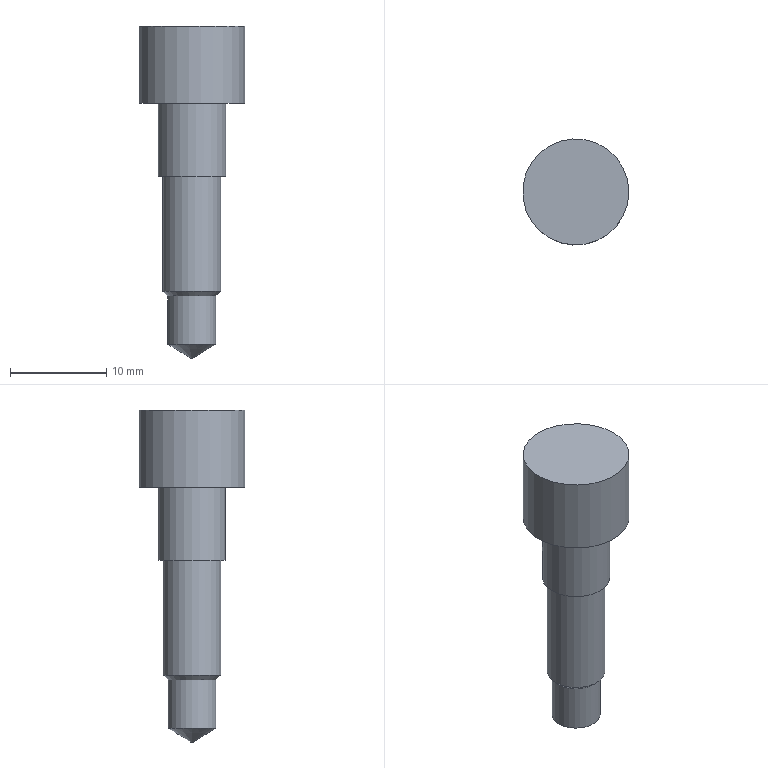Part | NX | features BREP 2 | 2 solids | 21 faces | box 11 x 11 x 34.43 mm | volume 2353 mm3 | plane 14 | cylinder 5 | cone 2 | commonest cylinder face diameters 5 x1 6 x1 7 x1 10 x1 11 x1
STEP:
#1=CARTESIAN_POINT('',(-2.5,0.,0.));
#2=VERTEX_POINT('',#1);
#3=CARTESIAN_POINT('',(0.,0.,0.));
#4=DIRECTION('',(0.,0.,1.));
#5=DIRECTION('',(-1.,0.,0.));
#6=AXIS2_PLACEMENT_3D('',#3,#4,#5);
#7=CIRCLE('',#6,2.5);
#8=EDGE_CURVE('',#2,#2,#7,.T.);
#9=ORIENTED_EDGE('',*,*,#8,.F.);
#10=EDGE_LOOP('',(#9));
#11=FACE_BOUND('',#10,.T.);
#12=CARTESIAN_POINT('',(-2.5,0.,-17.4));
#13=VERTEX_POINT('',#12);
#14=CARTESIAN_POINT('',(0.,0.,-17.4));
#15=DIRECTION('',(0.,0.,-1.));
#16=DIRECTION('',(-1.,0.,0.));
#17=AXIS2_PLACEMENT_3D('',#14,#15,#16);
#18=CIRCLE('',#17,2.5);
#19=EDGE_CURVE('',#13,#13,#18,.T.);
#20=ORIENTED_EDGE('',*,*,#19,.F.);
#21=EDGE_LOOP('',(#20));
#22=FACE_BOUND('',#21,.T.);
#23=CARTESIAN_POINT('',(0.,0.,-17.4));
#24=DIRECTION('',(0.,0.,1.));
#25=DIRECTION('',(-1.,0.,0.));
#26=AXIS2_PLACEMENT_3D('',#23,#24,#25);
#27=CYLINDRICAL_SURFACE('',#26,2.5);
#28=ADVANCED_FACE('',(#11,#22),#27,.T.);
#29=CARTESIAN_POINT('',(-0.1193,0.,-18.83));
#30=VERTEX_POINT('',#29);
#31=CARTESIAN_POINT('',(0.,0.,-18.83));
#32=DIRECTION('',(0.,0.,-1.));
#33=DIRECTION('',(-1.,0.,0.));
#34=AXIS2_PLACEMENT_3D('',#31,#32,#33);
#35=CIRCLE('',#34,0.1193);
#36=EDGE_CURVE('',#30,#30,#35,.T.);
#37=ORIENTED_EDGE('',*,*,#36,.T.);
#38=EDGE_LOOP('',(#37));
#39=FACE_BOUND('',#38,.T.);
#40=CARTESIAN_POINT('',(0.,0.,-18.83));
#41=DIRECTION('',(0.,0.,-1.));
#42=DIRECTION('',(1.,0.,0.));
#43=AXIS2_PLACEMENT_3D('',#40,#41,#42);
#44=PLANE('',#43);
#45=ADVANCED_FACE('',(#39),#44,.T.);
#46=ORIENTED_EDGE('',*,*,#36,.F.);
#47=EDGE_LOOP('',(#46));
#48=FACE_BOUND('',#47,.T.);
#49=ORIENTED_EDGE('',*,*,#19,.T.);
#50=EDGE_LOOP('',(#49));
#51=FACE_BOUND('',#50,.T.);
#52=CARTESIAN_POINT('',(0.,0.,-17.4));
#53=DIRECTION('',(0.,0.,1.));
#54=DIRECTION('',(-1.,0.,0.));
#55=AXIS2_PLACEMENT_3D('',#52,#53,#54);
#56=CONICAL_SURFACE('',#55,2.5,1.03);
#57=ADVANCED_FACE('',(#48,#51),#56,.T.);
#58=ORIENTED_EDGE('',*,*,#8,.T.);
#59=EDGE_LOOP('',(#58));
#60=FACE_BOUND('',#59,.T.);
#61=CARTESIAN_POINT('',(-3.5,0.,0.));
#62=VERTEX_POINT('',#61);
#63=CARTESIAN_POINT('',(0.,0.,0.));
#64=DIRECTION('',(0.,0.,-1.));
#65=DIRECTION('',(-1.,0.,0.));
#66=AXIS2_PLACEMENT_3D('',#63,#64,#65);
#67=CIRCLE('',#66,3.5);
#68=EDGE_CURVE('',#62,#62,#67,.T.);
#69=ORIENTED_EDGE('',*,*,#68,.T.);
#70=EDGE_LOOP('',(#69));
#71=FACE_BOUND('',#70,.T.);
#72=CARTESIAN_POINT('',(0.,0.,0.));
#73=DIRECTION('',(0.,0.,-1.));
#74=DIRECTION('',(1.,0.,0.));
#75=AXIS2_PLACEMENT_3D('',#72,#73,#74);
#76=PLANE('',#75);
#77=ADVANCED_FACE('',(#60,#71),#76,.T.);
#78=ORIENTED_EDGE('',*,*,#68,.F.);
#79=EDGE_LOOP('',(#78));
#80=FACE_BOUND('',#79,.T.);
#81=CARTESIAN_POINT('',(-3.5,0.,7.6));
#82=VERTEX_POINT('',#81);
#83=CARTESIAN_POINT('',(0.,0.,7.6));
#84=DIRECTION('',(0.,0.,-1.));
#85=DIRECTION('',(-1.,0.,0.));
#86=AXIS2_PLACEMENT_3D('',#83,#84,#85);
#87=CIRCLE('',#86,3.5);
#88=EDGE_CURVE('',#82,#82,#87,.T.);
#89=ORIENTED_EDGE('',*,*,#88,.T.);
#90=EDGE_LOOP('',(#89));
#91=FACE_BOUND('',#90,.T.);
#92=CARTESIAN_POINT('',(0.,0.,7.6));
#93=DIRECTION('',(0.,0.,-1.));
#94=DIRECTION('',(1.,0.,0.));
#95=AXIS2_PLACEMENT_3D('',#92,#93,#94);
#96=CYLINDRICAL_SURFACE('',#95,3.5);
#97=ADVANCED_FACE('',(#80,#91),#96,.T.);
#98=CARTESIAN_POINT('',(5.5,0.,15.6));
#99=VERTEX_POINT('',#98);
#100=CARTESIAN_POINT('',(0.,0.,15.6));
#101=DIRECTION('',(0.,0.,1.));
#102=DIRECTION('',(1.,0.,0.));
#103=AXIS2_PLACEMENT_3D('',#100,#101,#102);
#104=CIRCLE('',#103,5.5);
#105=EDGE_CURVE('',#99,#99,#104,.T.);
#106=ORIENTED_EDGE('',*,*,#105,.T.);
#107=EDGE_LOOP('',(#106));
#108=FACE_BOUND('',#107,.T.);
#109=CARTESIAN_POINT('',(0.,0.,15.6));
#110=DIRECTION('',(0.,0.,1.));
#111=DIRECTION('',(-1.,0.,0.));
#112=AXIS2_PLACEMENT_3D('',#109,#110,#111);
#113=PLANE('',#112);
#114=ADVANCED_FACE('',(#108),#113,.T.);
#115=ORIENTED_EDGE('',*,*,#105,.F.);
#116=EDGE_LOOP('',(#115));
#117=FACE_BOUND('',#116,.T.);
#118=CARTESIAN_POINT('',(5.5,0.,7.6));
#119=VERTEX_POINT('',#118);
#120=CARTESIAN_POINT('',(0.,0.,7.6));
#121=DIRECTION('',(0.,0.,1.));
#122=DIRECTION('',(1.,0.,0.));
#123=AXIS2_PLACEMENT_3D('',#120,#121,#122);
#124=CIRCLE('',#123,5.5);
#125=EDGE_CURVE('',#119,#119,#124,.T.);
#126=ORIENTED_EDGE('',*,*,#125,.T.);
#127=EDGE_LOOP('',(#126));
#128=FACE_BOUND('',#127,.T.);
#129=CARTESIAN_POINT('',(0.,0.,7.6));
#130=DIRECTION('',(0.,0.,1.));
#131=DIRECTION('',(-1.,0.,0.));
#132=AXIS2_PLACEMENT_3D('',#129,#130,#131);
#133=CYLINDRICAL_SURFACE('',#132,5.5);
#134=ADVANCED_FACE('',(#117,#128),#133,.T.);
#135=ORIENTED_EDGE('',*,*,#88,.F.);
#136=EDGE_LOOP('',(#135));
#137=FACE_BOUND('',#136,.T.);
#138=ORIENTED_EDGE('',*,*,#125,.F.);
#139=EDGE_LOOP('',(#138));
#140=FACE_BOUND('',#139,.T.);
#141=CARTESIAN_POINT('',(0.,0.,7.6));
#142=DIRECTION('',(0.,0.,-1.));
#143=DIRECTION('',(1.,0.,0.));
#144=AXIS2_PLACEMENT_3D('',#141,#142,#143);
#145=PLANE('',#144);
#146=ADVANCED_FACE('',(#137,#140),#145,.T.);
#147=CLOSED_SHELL('',(#28,#45,#57,#77,#97,#114,#134,#146));
#148=MANIFOLD_SOLID_BREP('',#147);
#149=CARTESIAN_POINT('',(5.,0.,13.6));
#150=VERTEX_POINT('',#149);
#151=CARTESIAN_POINT('',(0.,0.,13.6));
#152=DIRECTION('',(0.,0.,1.));
#153=DIRECTION('',(1.,0.,0.));
#154=AXIS2_PLACEMENT_3D('',#151,#152,#153);
#155=CIRCLE('',#154,5.);
#156=EDGE_CURVE('',#150,#150,#155,.T.);
#157=ORIENTED_EDGE('',*,*,#156,.T.);
#158=EDGE_LOOP('',(#157));
#159=FACE_BOUND('',#158,.T.);
#160=CARTESIAN_POINT('',(2.887,0.,13.6));
#161=VERTEX_POINT('',#160);
#162=CARTESIAN_POINT('',(1.443,-2.5,13.6));
#163=VERTEX_POINT('',#162);
#164=CARTESIAN_POINT('',(2.887,0.,13.6));
#165=DIRECTION('',(-0.5,-0.866,0.));
#166=VECTOR('',#165,1000.);
#167=LINE('',#164,#166);
#168=EDGE_CURVE('',#161,#163,#167,.T.);
#169=ORIENTED_EDGE('',*,*,#168,.T.);
#170=CARTESIAN_POINT('',(-1.443,-2.5,13.6));
#171=VERTEX_POINT('',#170);
#172=CARTESIAN_POINT('',(1.443,-2.5,13.6));
#173=DIRECTION('',(-1.,0.,0.));
#174=VECTOR('',#173,1000.);
#175=LINE('',#172,#174);
#176=EDGE_CURVE('',#163,#171,#175,.T.);
#177=ORIENTED_EDGE('',*,*,#176,.T.);
#178=CARTESIAN_POINT('',(-2.887,0.,13.6));
#179=VERTEX_POINT('',#178);
#180=CARTESIAN_POINT('',(-1.443,-2.5,13.6));
#181=DIRECTION('',(-0.5,0.866,0.));
#182=VECTOR('',#181,1000.);
#183=LINE('',#180,#182);
#184=EDGE_CURVE('',#171,#179,#183,.T.);
#185=ORIENTED_EDGE('',*,*,#184,.T.);
#186=CARTESIAN_POINT('',(-1.443,2.5,13.6));
#187=VERTEX_POINT('',#186);
#188=CARTESIAN_POINT('',(-2.887,0.,13.6));
#189=DIRECTION('',(0.5,0.866,0.));
#190=VECTOR('',#189,1000.);
#191=LINE('',#188,#190);
#192=EDGE_CURVE('',#179,#187,#191,.T.);
#193=ORIENTED_EDGE('',*,*,#192,.T.);
#194=CARTESIAN_POINT('',(1.443,2.5,13.6));
#195=VERTEX_POINT('',#194);
#196=CARTESIAN_POINT('',(-1.443,2.5,13.6));
#197=DIRECTION('',(1.,0.,0.));
#198=VECTOR('',#197,1000.);
#199=LINE('',#196,#198);
#200=EDGE_CURVE('',#187,#195,#199,.T.);
#201=ORIENTED_EDGE('',*,*,#200,.T.);
#202=CARTESIAN_POINT('',(1.443,2.5,13.6));
#203=DIRECTION('',(0.5,-0.866,0.));
#204=VECTOR('',#203,1000.);
#205=LINE('',#202,#204);
#206=EDGE_CURVE('',#195,#161,#205,.T.);
#207=ORIENTED_EDGE('',*,*,#206,.T.);
#208=EDGE_LOOP('',(#169,#177,#185,#193,#201,#207));
#209=FACE_BOUND('',#208,.T.);
#210=CARTESIAN_POINT('',(0.,0.,13.6));
#211=DIRECTION('',(0.,0.,1.));
#212=DIRECTION('',(-1.,0.,0.));
#213=AXIS2_PLACEMENT_3D('',#210,#211,#212);
#214=PLANE('',#213);
#215=ADVANCED_FACE('',(#159,#209),#214,.T.);
#216=CARTESIAN_POINT('',(3.,0.,-11.9));
#217=VERTEX_POINT('',#216);
#218=CARTESIAN_POINT('',(0.,0.,-11.9));
#219=DIRECTION('',(0.,0.,1.));
#220=DIRECTION('',(1.,0.,0.));
#221=AXIS2_PLACEMENT_3D('',#218,#219,#220);
#222=CIRCLE('',#221,3.);
#223=EDGE_CURVE('',#217,#217,#222,.T.);
#224=ORIENTED_EDGE('',*,*,#223,.T.);
#225=EDGE_LOOP('',(#224));
#226=FACE_BOUND('',#225,.T.);
#227=CARTESIAN_POINT('',(3.,0.,7.6));
#228=VERTEX_POINT('',#227);
#229=CARTESIAN_POINT('',(0.,0.,7.6));
#230=DIRECTION('',(0.,0.,1.));
#231=DIRECTION('',(1.,0.,0.));
#232=AXIS2_PLACEMENT_3D('',#229,#230,#231);
#233=CIRCLE('',#232,3.);
#234=EDGE_CURVE('',#228,#228,#233,.T.);
#235=ORIENTED_EDGE('',*,*,#234,.F.);
#236=EDGE_LOOP('',(#235));
#237=FACE_BOUND('',#236,.T.);
#238=CARTESIAN_POINT('',(0.,0.,-12.4));
#239=DIRECTION('',(0.,0.,1.));
#240=DIRECTION('',(-1.,0.,0.));
#241=AXIS2_PLACEMENT_3D('',#238,#239,#240);
#242=CYLINDRICAL_SURFACE('',#241,3.);
#243=ADVANCED_FACE('',(#226,#237),#242,.T.);
#244=CARTESIAN_POINT('',(2.5,0.,-12.4));
#245=VERTEX_POINT('',#244);
#246=CARTESIAN_POINT('',(0.,0.,-12.4));
#247=DIRECTION('',(0.,0.,-1.));
#248=DIRECTION('',(1.,0.,0.));
#249=AXIS2_PLACEMENT_3D('',#246,#247,#248);
#250=CIRCLE('',#249,2.5);
#251=EDGE_CURVE('',#245,#245,#250,.T.);
#252=ORIENTED_EDGE('',*,*,#251,.T.);
#253=EDGE_LOOP('',(#252));
#254=FACE_BOUND('',#253,.T.);
#255=CARTESIAN_POINT('',(0.,0.,-12.4));
#256=DIRECTION('',(0.,0.,1.));
#257=DIRECTION('',(-1.,0.,0.));
#258=AXIS2_PLACEMENT_3D('',#255,#256,#257);
#259=PLANE('',#258);
#260=ADVANCED_FACE('',(#254),#259,.F.);
#261=ORIENTED_EDGE('',*,*,#234,.T.);
#262=EDGE_LOOP('',(#261));
#263=FACE_BOUND('',#262,.T.);
#264=CARTESIAN_POINT('',(5.,0.,7.6));
#265=VERTEX_POINT('',#264);
#266=CARTESIAN_POINT('',(0.,0.,7.6));
#267=DIRECTION('',(0.,0.,1.));
#268=DIRECTION('',(1.,0.,0.));
#269=AXIS2_PLACEMENT_3D('',#266,#267,#268);
#270=CIRCLE('',#269,5.);
#271=EDGE_CURVE('',#265,#265,#270,.T.);
#272=ORIENTED_EDGE('',*,*,#271,.F.);
#273=EDGE_LOOP('',(#272));
#274=FACE_BOUND('',#273,.T.);
#275=CARTESIAN_POINT('',(0.,0.,7.6));
#276=DIRECTION('',(0.,0.,-1.));
#277=DIRECTION('',(1.,0.,0.));
#278=AXIS2_PLACEMENT_3D('',#275,#276,#277);
#279=PLANE('',#278);
#280=ADVANCED_FACE('',(#263,#274),#279,.T.);
#281=ORIENTED_EDGE('',*,*,#156,.F.);
#282=EDGE_LOOP('',(#281));
#283=FACE_BOUND('',#282,.T.);
#284=ORIENTED_EDGE('',*,*,#271,.T.);
#285=EDGE_LOOP('',(#284));
#286=FACE_BOUND('',#285,.T.);
#287=CARTESIAN_POINT('',(0.,0.,7.6));
#288=DIRECTION('',(0.,0.,1.));
#289=DIRECTION('',(-1.,0.,0.));
#290=AXIS2_PLACEMENT_3D('',#287,#288,#289);
#291=CYLINDRICAL_SURFACE('',#290,5.);
#292=ADVANCED_FACE('',(#283,#286),#291,.T.);
#293=ORIENTED_EDGE('',*,*,#251,.F.);
#294=EDGE_LOOP('',(#293));
#295=FACE_BOUND('',#294,.T.);
#296=ORIENTED_EDGE('',*,*,#223,.F.);
#297=EDGE_LOOP('',(#296));
#298=FACE_BOUND('',#297,.T.);
#299=CARTESIAN_POINT('',(0.,0.,-11.9));
#300=DIRECTION('',(0.,0.,1.));
#301=DIRECTION('',(-1.,0.,0.));
#302=AXIS2_PLACEMENT_3D('',#299,#300,#301);
#303=CONICAL_SURFACE('',#302,3.,0.7854);
#304=ADVANCED_FACE('',(#295,#298),#303,.T.);
#305=ORIENTED_EDGE('',*,*,#176,.F.);
#306=CARTESIAN_POINT('',(1.443,-2.5,9.64));
#307=VERTEX_POINT('',#306);
#308=CARTESIAN_POINT('',(1.443,-2.5,9.64));
#309=DIRECTION('',(0.,0.,1.));
#310=VECTOR('',#309,1000.);
#311=LINE('',#308,#310);
#312=EDGE_CURVE('',#307,#163,#311,.T.);
#313=ORIENTED_EDGE('',*,*,#312,.F.);
#314=CARTESIAN_POINT('',(-1.443,-2.5,9.64));
#315=VERTEX_POINT('',#314);
#316=CARTESIAN_POINT('',(1.443,-2.5,9.64));
#317=DIRECTION('',(-1.,0.,0.));
#318=VECTOR('',#317,1000.);
#319=LINE('',#316,#318);
#320=EDGE_CURVE('',#307,#315,#319,.T.);
#321=ORIENTED_EDGE('',*,*,#320,.T.);
#322=CARTESIAN_POINT('',(-1.443,-2.5,9.64));
#323=DIRECTION('',(0.,0.,1.));
#324=VECTOR('',#323,1000.);
#325=LINE('',#322,#324);
#326=EDGE_CURVE('',#315,#171,#325,.T.);
#327=ORIENTED_EDGE('',*,*,#326,.T.);
#328=EDGE_LOOP('',(#305,#313,#321,#327));
#329=FACE_BOUND('',#328,.T.);
#330=CARTESIAN_POINT('',(1.443,-2.5,9.64));
#331=DIRECTION('',(0.,1.,0.));
#332=DIRECTION('',(0.,0.,-1.));
#333=AXIS2_PLACEMENT_3D('',#330,#331,#332);
#334=PLANE('',#333);
#335=ADVANCED_FACE('',(#329),#334,.T.);
#336=ORIENTED_EDGE('',*,*,#184,.F.);
#337=ORIENTED_EDGE('',*,*,#326,.F.);
#338=CARTESIAN_POINT('',(-2.887,0.,9.64));
#339=VERTEX_POINT('',#338);
#340=CARTESIAN_POINT('',(-1.443,-2.5,9.64));
#341=DIRECTION('',(-0.5,0.866,0.));
#342=VECTOR('',#341,1000.);
#343=LINE('',#340,#342);
#344=EDGE_CURVE('',#315,#339,#343,.T.);
#345=ORIENTED_EDGE('',*,*,#344,.T.);
#346=CARTESIAN_POINT('',(-2.887,0.,9.64));
#347=DIRECTION('',(0.,0.,1.));
#348=VECTOR('',#347,1000.);
#349=LINE('',#346,#348);
#350=EDGE_CURVE('',#339,#179,#349,.T.);
#351=ORIENTED_EDGE('',*,*,#350,.T.);
#352=EDGE_LOOP('',(#336,#337,#345,#351));
#353=FACE_BOUND('',#352,.T.);
#354=CARTESIAN_POINT('',(-1.443,-2.5,9.64));
#355=DIRECTION('',(0.866,0.5,0.));
#356=DIRECTION('',(0.5,-0.866,0.));
#357=AXIS2_PLACEMENT_3D('',#354,#355,#356);
#358=PLANE('',#357);
#359=ADVANCED_FACE('',(#353),#358,.T.);
#360=ORIENTED_EDGE('',*,*,#192,.F.);
#361=ORIENTED_EDGE('',*,*,#350,.F.);
#362=CARTESIAN_POINT('',(-1.443,2.5,9.64));
#363=VERTEX_POINT('',#362);
#364=CARTESIAN_POINT('',(-2.887,0.,9.64));
#365=DIRECTION('',(0.5,0.866,0.));
#366=VECTOR('',#365,1000.);
#367=LINE('',#364,#366);
#368=EDGE_CURVE('',#339,#363,#367,.T.);
#369=ORIENTED_EDGE('',*,*,#368,.T.);
#370=CARTESIAN_POINT('',(-1.443,2.5,9.64));
#371=DIRECTION('',(0.,0.,1.));
#372=VECTOR('',#371,1000.);
#373=LINE('',#370,#372);
#374=EDGE_CURVE('',#363,#187,#373,.T.);
#375=ORIENTED_EDGE('',*,*,#374,.T.);
#376=EDGE_LOOP('',(#360,#361,#369,#375));
#377=FACE_BOUND('',#376,.T.);
#378=CARTESIAN_POINT('',(-2.887,0.,9.64));
#379=DIRECTION('',(0.866,-0.5,0.));
#380=DIRECTION('',(-0.5,-0.866,0.));
#381=AXIS2_PLACEMENT_3D('',#378,#379,#380);
#382=PLANE('',#381);
#383=ADVANCED_FACE('',(#377),#382,.T.);
#384=ORIENTED_EDGE('',*,*,#200,.F.);
#385=ORIENTED_EDGE('',*,*,#374,.F.);
#386=CARTESIAN_POINT('',(1.443,2.5,9.64));
#387=VERTEX_POINT('',#386);
#388=CARTESIAN_POINT('',(-1.443,2.5,9.64));
#389=DIRECTION('',(1.,0.,0.));
#390=VECTOR('',#389,1000.);
#391=LINE('',#388,#390);
#392=EDGE_CURVE('',#363,#387,#391,.T.);
#393=ORIENTED_EDGE('',*,*,#392,.T.);
#394=CARTESIAN_POINT('',(1.443,2.5,9.64));
#395=DIRECTION('',(0.,0.,1.));
#396=VECTOR('',#395,1000.);
#397=LINE('',#394,#396);
#398=EDGE_CURVE('',#387,#195,#397,.T.);
#399=ORIENTED_EDGE('',*,*,#398,.T.);
#400=EDGE_LOOP('',(#384,#385,#393,#399));
#401=FACE_BOUND('',#400,.T.);
#402=CARTESIAN_POINT('',(-1.443,2.5,9.64));
#403=DIRECTION('',(0.,-1.,0.));
#404=DIRECTION('',(0.,0.,1.));
#405=AXIS2_PLACEMENT_3D('',#402,#403,#404);
#406=PLANE('',#405);
#407=ADVANCED_FACE('',(#401),#406,.T.);
#408=ORIENTED_EDGE('',*,*,#206,.F.);
#409=ORIENTED_EDGE('',*,*,#398,.F.);
#410=CARTESIAN_POINT('',(2.887,0.,9.64));
#411=VERTEX_POINT('',#410);
#412=CARTESIAN_POINT('',(1.443,2.5,9.64));
#413=DIRECTION('',(0.5,-0.866,0.));
#414=VECTOR('',#413,1000.);
#415=LINE('',#412,#414);
#416=EDGE_CURVE('',#387,#411,#415,.T.);
#417=ORIENTED_EDGE('',*,*,#416,.T.);
#418=CARTESIAN_POINT('',(2.887,0.,9.64));
#419=DIRECTION('',(0.,0.,1.));
#420=VECTOR('',#419,1000.);
#421=LINE('',#418,#420);
#422=EDGE_CURVE('',#411,#161,#421,.T.);
#423=ORIENTED_EDGE('',*,*,#422,.T.);
#424=EDGE_LOOP('',(#408,#409,#417,#423));
#425=FACE_BOUND('',#424,.T.);
#426=CARTESIAN_POINT('',(1.443,2.5,9.64));
#427=DIRECTION('',(-0.866,-0.5,0.));
#428=DIRECTION('',(-0.5,0.866,0.));
#429=AXIS2_PLACEMENT_3D('',#426,#427,#428);
#430=PLANE('',#429);
#431=ADVANCED_FACE('',(#425),#430,.T.);
#432=ORIENTED_EDGE('',*,*,#168,.F.);
#433=ORIENTED_EDGE('',*,*,#422,.F.);
#434=CARTESIAN_POINT('',(2.887,0.,9.64));
#435=DIRECTION('',(-0.5,-0.866,0.));
#436=VECTOR('',#435,1000.);
#437=LINE('',#434,#436);
#438=EDGE_CURVE('',#411,#307,#437,.T.);
#439=ORIENTED_EDGE('',*,*,#438,.T.);
#440=ORIENTED_EDGE('',*,*,#312,.T.);
#441=EDGE_LOOP('',(#432,#433,#439,#440));
#442=FACE_BOUND('',#441,.T.);
#443=CARTESIAN_POINT('',(2.887,0.,9.64));
#444=DIRECTION('',(-0.866,0.5,0.));
#445=DIRECTION('',(0.5,0.866,0.));
#446=AXIS2_PLACEMENT_3D('',#443,#444,#445);
#447=PLANE('',#446);
#448=ADVANCED_FACE('',(#442),#447,.T.);
#449=ORIENTED_EDGE('',*,*,#320,.F.);
#450=ORIENTED_EDGE('',*,*,#438,.F.);
#451=ORIENTED_EDGE('',*,*,#416,.F.);
#452=ORIENTED_EDGE('',*,*,#392,.F.);
#453=ORIENTED_EDGE('',*,*,#368,.F.);
#454=ORIENTED_EDGE('',*,*,#344,.F.);
#455=EDGE_LOOP('',(#449,#450,#451,#452,#453,#454));
#456=FACE_BOUND('',#455,.T.);
#457=CARTESIAN_POINT('',(-4.33,-2.5,9.64));
#458=DIRECTION('',(0.,0.,-1.));
#459=DIRECTION('',(1.,0.,0.));
#460=AXIS2_PLACEMENT_3D('',#457,#458,#459);
#461=PLANE('',#460);
#462=ADVANCED_FACE('',(#456),#461,.F.);
#463=CLOSED_SHELL('',(#215,#243,#260,#280,#292,#304,#335,#359,#383,#407,#431,#448,#462));
#464=MANIFOLD_SOLID_BREP('',#463);
#465=(LENGTH_UNIT()NAMED_UNIT(*)SI_UNIT(.MILLI.,.METRE.));
#466=UNCERTAINTY_MEASURE_WITH_UNIT(LENGTH_MEASURE(0.00001),#465,'','');
#467=(NAMED_UNIT(*)PLANE_ANGLE_UNIT()SI_UNIT($,.RADIAN.));
#468=(NAMED_UNIT(*)SI_UNIT($,.STERADIAN.)SOLID_ANGLE_UNIT());
#469=(GEOMETRIC_REPRESENTATION_CONTEXT(3)GLOBAL_UNCERTAINTY_ASSIGNED_CONTEXT((#466))GLOBAL_UNIT_ASSIGNED_CONTEXT((#465,#467,#468))REPRESENTATION_CONTEXT('',''));
#470=ADVANCED_BREP_SHAPE_REPRESENTATION('',(#148,#464),#469);